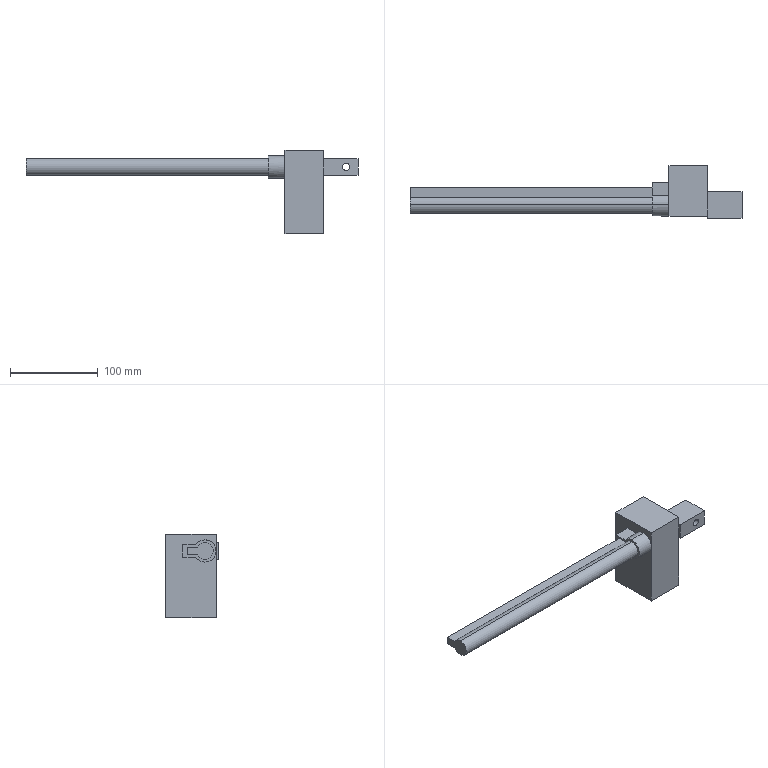Part | NX | features BREP 1 | 1 solid | 28 faces | box 379 x 59.436 x 95.25 mm | volume 383836 mm3 | plane 20 | cylinder 8 | commonest cylinder face diameters 19.304 x3 25.4 x3 8.255 x2
STEP:
#1=CARTESIAN_POINT('',(-19.05,25.4,6.985));
#2=VERTEX_POINT('',#1);
#3=CARTESIAN_POINT('',(-19.05,25.4,-6.985));
#4=VERTEX_POINT('',#3);
#5=CARTESIAN_POINT('',(-19.05,25.4,6.985));
#6=DIRECTION('',(0.,0.,-1.));
#7=VECTOR('',#6,1000.);
#8=LINE('',#5,#7);
#9=EDGE_CURVE('',#2,#4,#8,.T.);
#10=ORIENTED_EDGE('',*,*,#9,.T.);
#11=CARTESIAN_POINT('',(-19.05,10.607,-6.985));
#12=VERTEX_POINT('',#11);
#13=CARTESIAN_POINT('',(-19.05,25.4,-6.985));
#14=DIRECTION('',(0.,-1.,0.));
#15=VECTOR('',#14,1000.);
#16=LINE('',#13,#15);
#17=EDGE_CURVE('',#4,#12,#16,.T.);
#18=ORIENTED_EDGE('',*,*,#17,.T.);
#19=CARTESIAN_POINT('',(-19.05,0.,-12.7));
#20=VERTEX_POINT('',#19);
#21=CARTESIAN_POINT('',(-19.05,0.,0.));
#22=DIRECTION('',(-1.,0.,0.));
#23=DIRECTION('',(0.,0.8352,-0.55));
#24=AXIS2_PLACEMENT_3D('',#21,#22,#23);
#25=CIRCLE('',#24,12.7);
#26=EDGE_CURVE('',#12,#20,#25,.T.);
#27=ORIENTED_EDGE('',*,*,#26,.T.);
#28=CARTESIAN_POINT('',(-19.05,0.,12.7));
#29=VERTEX_POINT('',#28);
#30=CARTESIAN_POINT('',(-19.05,0.,0.));
#31=DIRECTION('',(-1.,0.,0.));
#32=DIRECTION('',(0.,0.8352,-0.55));
#33=AXIS2_PLACEMENT_3D('',#30,#31,#32);
#34=CIRCLE('',#33,12.7);
#35=EDGE_CURVE('',#20,#29,#34,.T.);
#36=ORIENTED_EDGE('',*,*,#35,.T.);
#37=CARTESIAN_POINT('',(-19.05,10.607,6.985));
#38=VERTEX_POINT('',#37);
#39=CARTESIAN_POINT('',(-19.05,0.,0.));
#40=DIRECTION('',(-1.,0.,0.));
#41=DIRECTION('',(0.,0.8352,-0.55));
#42=AXIS2_PLACEMENT_3D('',#39,#40,#41);
#43=CIRCLE('',#42,12.7);
#44=EDGE_CURVE('',#29,#38,#43,.T.);
#45=ORIENTED_EDGE('',*,*,#44,.T.);
#46=CARTESIAN_POINT('',(-19.05,10.607,6.985));
#47=DIRECTION('',(0.,1.,0.));
#48=VECTOR('',#47,1000.);
#49=LINE('',#46,#48);
#50=EDGE_CURVE('',#38,#2,#49,.T.);
#51=ORIENTED_EDGE('',*,*,#50,.T.);
#52=EDGE_LOOP('',(#10,#18,#27,#36,#45,#51));
#53=FACE_BOUND('',#52,.T.);
#54=CARTESIAN_POINT('',(-19.05,20.32,4.445));
#55=VERTEX_POINT('',#54);
#56=CARTESIAN_POINT('',(-19.05,20.32,-4.445));
#57=VERTEX_POINT('',#56);
#58=CARTESIAN_POINT('',(-19.05,20.32,4.445));
#59=DIRECTION('',(0.,0.,-1.));
#60=VECTOR('',#59,1000.);
#61=LINE('',#58,#60);
#62=EDGE_CURVE('',#55,#57,#61,.T.);
#63=ORIENTED_EDGE('',*,*,#62,.F.);
#64=CARTESIAN_POINT('',(-19.05,8.568,4.445));
#65=VERTEX_POINT('',#64);
#66=CARTESIAN_POINT('',(-19.05,8.568,4.445));
#67=DIRECTION('',(0.,1.,0.));
#68=VECTOR('',#67,1000.);
#69=LINE('',#66,#68);
#70=EDGE_CURVE('',#65,#55,#69,.T.);
#71=ORIENTED_EDGE('',*,*,#70,.F.);
#72=CARTESIAN_POINT('',(-19.05,0.,9.652));
#73=VERTEX_POINT('',#72);
#74=CARTESIAN_POINT('',(-19.05,0.,0.));
#75=DIRECTION('',(-1.,0.,0.));
#76=DIRECTION('',(0.,0.8876,-0.4605));
#77=AXIS2_PLACEMENT_3D('',#74,#75,#76);
#78=CIRCLE('',#77,9.652);
#79=EDGE_CURVE('',#73,#65,#78,.T.);
#80=ORIENTED_EDGE('',*,*,#79,.F.);
#81=CARTESIAN_POINT('',(-19.05,0.,-9.652));
#82=VERTEX_POINT('',#81);
#83=CARTESIAN_POINT('',(-19.05,0.,0.));
#84=DIRECTION('',(-1.,0.,0.));
#85=DIRECTION('',(0.,0.8876,-0.4605));
#86=AXIS2_PLACEMENT_3D('',#83,#84,#85);
#87=CIRCLE('',#86,9.652);
#88=EDGE_CURVE('',#82,#73,#87,.T.);
#89=ORIENTED_EDGE('',*,*,#88,.F.);
#90=CARTESIAN_POINT('',(-19.05,8.568,-4.445));
#91=VERTEX_POINT('',#90);
#92=CARTESIAN_POINT('',(-19.05,0.,0.));
#93=DIRECTION('',(-1.,0.,0.));
#94=DIRECTION('',(0.,0.8876,-0.4605));
#95=AXIS2_PLACEMENT_3D('',#92,#93,#94);
#96=CIRCLE('',#95,9.652);
#97=EDGE_CURVE('',#91,#82,#96,.T.);
#98=ORIENTED_EDGE('',*,*,#97,.F.);
#99=CARTESIAN_POINT('',(-19.05,20.32,-4.445));
#100=DIRECTION('',(0.,-1.,0.));
#101=VECTOR('',#100,1000.);
#102=LINE('',#99,#101);
#103=EDGE_CURVE('',#57,#91,#102,.T.);
#104=ORIENTED_EDGE('',*,*,#103,.F.);
#105=EDGE_LOOP('',(#63,#71,#80,#89,#98,#104));
#106=FACE_BOUND('',#105,.T.);
#107=CARTESIAN_POINT('',(-19.05,0.,0.));
#108=DIRECTION('',(1.,0.,0.));
#109=DIRECTION('',(0.,1.,0.));
#110=AXIS2_PLACEMENT_3D('',#107,#108,#109);
#111=PLANE('',#110);
#112=ADVANCED_FACE('',(#53,#106),#111,.F.);
#113=CARTESIAN_POINT('',(0.,25.4,6.985));
#114=VERTEX_POINT('',#113);
#115=CARTESIAN_POINT('',(-19.05,25.4,6.985));
#116=DIRECTION('',(1.,0.,0.));
#117=VECTOR('',#116,1000.);
#118=LINE('',#115,#117);
#119=EDGE_CURVE('',#2,#114,#118,.T.);
#120=ORIENTED_EDGE('',*,*,#119,.F.);
#121=ORIENTED_EDGE('',*,*,#50,.F.);
#122=CARTESIAN_POINT('',(0.,10.607,6.985));
#123=VERTEX_POINT('',#122);
#124=CARTESIAN_POINT('',(-19.05,10.607,6.985));
#125=DIRECTION('',(1.,0.,0.));
#126=VECTOR('',#125,1000.);
#127=LINE('',#124,#126);
#128=EDGE_CURVE('',#38,#123,#127,.T.);
#129=ORIENTED_EDGE('',*,*,#128,.T.);
#130=CARTESIAN_POINT('',(0.,25.4,6.985));
#131=DIRECTION('',(0.,-1.,0.));
#132=VECTOR('',#131,1000.);
#133=LINE('',#130,#132);
#134=EDGE_CURVE('',#114,#123,#133,.T.);
#135=ORIENTED_EDGE('',*,*,#134,.F.);
#136=EDGE_LOOP('',(#120,#121,#129,#135));
#137=FACE_BOUND('',#136,.T.);
#138=CARTESIAN_POINT('',(0.,25.4,6.985));
#139=DIRECTION('',(0.,0.,1.));
#140=DIRECTION('',(1.,0.,0.));
#141=AXIS2_PLACEMENT_3D('',#138,#139,#140);
#142=PLANE('',#141);
#143=ADVANCED_FACE('',(#137),#142,.T.);
#144=CARTESIAN_POINT('',(0.,0.,12.7));
#145=VERTEX_POINT('',#144);
#146=CARTESIAN_POINT('',(0.,0.,0.));
#147=DIRECTION('',(1.,0.,0.));
#148=DIRECTION('',(0.,0.8352,0.55));
#149=AXIS2_PLACEMENT_3D('',#146,#147,#148);
#150=CIRCLE('',#149,12.7);
#151=EDGE_CURVE('',#123,#145,#150,.T.);
#152=ORIENTED_EDGE('',*,*,#151,.T.);
#153=CARTESIAN_POINT('',(0.,-12.7,0.));
#154=VERTEX_POINT('',#153);
#155=CARTESIAN_POINT('',(0.,0.,0.));
#156=DIRECTION('',(1.,0.,0.));
#157=DIRECTION('',(0.,0.8352,0.55));
#158=AXIS2_PLACEMENT_3D('',#155,#156,#157);
#159=CIRCLE('',#158,12.7);
#160=EDGE_CURVE('',#145,#154,#159,.T.);
#161=ORIENTED_EDGE('',*,*,#160,.T.);
#162=CARTESIAN_POINT('',(0.,-12.7,19.05));
#163=VERTEX_POINT('',#162);
#164=CARTESIAN_POINT('',(0.,-12.7,0.));
#165=DIRECTION('',(0.,0.,1.));
#166=VECTOR('',#165,1000.);
#167=LINE('',#164,#166);
#168=EDGE_CURVE('',#154,#163,#167,.T.);
#169=ORIENTED_EDGE('',*,*,#168,.T.);
#170=CARTESIAN_POINT('',(0.,44.45,19.05));
#171=VERTEX_POINT('',#170);
#172=CARTESIAN_POINT('',(0.,44.45,19.05));
#173=DIRECTION('',(0.,-1.,0.));
#174=VECTOR('',#173,1000.);
#175=LINE('',#172,#174);
#176=EDGE_CURVE('',#171,#163,#175,.T.);
#177=ORIENTED_EDGE('',*,*,#176,.F.);
#178=CARTESIAN_POINT('',(0.,44.45,-76.2));
#179=VERTEX_POINT('',#178);
#180=CARTESIAN_POINT('',(0.,44.45,-76.2));
#181=DIRECTION('',(0.,0.,1.));
#182=VECTOR('',#181,1000.);
#183=LINE('',#180,#182);
#184=EDGE_CURVE('',#179,#171,#183,.T.);
#185=ORIENTED_EDGE('',*,*,#184,.F.);
#186=CARTESIAN_POINT('',(0.,-12.7,-76.2));
#187=VERTEX_POINT('',#186);
#188=CARTESIAN_POINT('',(0.,44.45,-76.2));
#189=DIRECTION('',(0.,-1.,0.));
#190=VECTOR('',#189,1000.);
#191=LINE('',#188,#190);
#192=EDGE_CURVE('',#179,#187,#191,.T.);
#193=ORIENTED_EDGE('',*,*,#192,.T.);
#194=CARTESIAN_POINT('',(0.,-12.7,-76.2));
#195=DIRECTION('',(0.,0.,1.));
#196=VECTOR('',#195,1000.);
#197=LINE('',#194,#196);
#198=EDGE_CURVE('',#187,#154,#197,.T.);
#199=ORIENTED_EDGE('',*,*,#198,.T.);
#200=CARTESIAN_POINT('',(0.,0.,-12.7));
#201=VERTEX_POINT('',#200);
#202=CARTESIAN_POINT('',(0.,0.,0.));
#203=DIRECTION('',(1.,0.,0.));
#204=DIRECTION('',(0.,-1.,0.));
#205=AXIS2_PLACEMENT_3D('',#202,#203,#204);
#206=CIRCLE('',#205,12.7);
#207=EDGE_CURVE('',#154,#201,#206,.T.);
#208=ORIENTED_EDGE('',*,*,#207,.T.);
#209=CARTESIAN_POINT('',(0.,10.607,-6.985));
#210=VERTEX_POINT('',#209);
#211=CARTESIAN_POINT('',(0.,0.,0.));
#212=DIRECTION('',(1.,0.,0.));
#213=DIRECTION('',(0.,-1.,0.));
#214=AXIS2_PLACEMENT_3D('',#211,#212,#213);
#215=CIRCLE('',#214,12.7);
#216=EDGE_CURVE('',#201,#210,#215,.T.);
#217=ORIENTED_EDGE('',*,*,#216,.T.);
#218=CARTESIAN_POINT('',(0.,25.4,-6.985));
#219=VERTEX_POINT('',#218);
#220=CARTESIAN_POINT('',(0.,10.607,-6.985));
#221=DIRECTION('',(0.,1.,0.));
#222=VECTOR('',#221,1000.);
#223=LINE('',#220,#222);
#224=EDGE_CURVE('',#210,#219,#223,.T.);
#225=ORIENTED_EDGE('',*,*,#224,.T.);
#226=CARTESIAN_POINT('',(0.,25.4,-6.985));
#227=DIRECTION('',(0.,0.,1.));
#228=VECTOR('',#227,1000.);
#229=LINE('',#226,#228);
#230=EDGE_CURVE('',#219,#114,#229,.T.);
#231=ORIENTED_EDGE('',*,*,#230,.T.);
#232=ORIENTED_EDGE('',*,*,#134,.T.);
#233=EDGE_LOOP('',(#152,#161,#169,#177,#185,#193,#199,#208,#217,#225,#231,#232));
#234=FACE_BOUND('',#233,.T.);
#235=CARTESIAN_POINT('',(0.,44.45,-76.2));
#236=DIRECTION('',(-1.,0.,0.));
#237=DIRECTION('',(0.,0.,1.));
#238=AXIS2_PLACEMENT_3D('',#235,#236,#237);
#239=PLANE('',#238);
#240=ADVANCED_FACE('',(#234),#239,.T.);
#241=CARTESIAN_POINT('',(-19.05,25.4,-6.985));
#242=DIRECTION('',(1.,0.,0.));
#243=VECTOR('',#242,1000.);
#244=LINE('',#241,#243);
#245=EDGE_CURVE('',#4,#219,#244,.T.);
#246=ORIENTED_EDGE('',*,*,#245,.F.);
#247=ORIENTED_EDGE('',*,*,#9,.F.);
#248=ORIENTED_EDGE('',*,*,#119,.T.);
#249=ORIENTED_EDGE('',*,*,#230,.F.);
#250=EDGE_LOOP('',(#246,#247,#248,#249));
#251=FACE_BOUND('',#250,.T.);
#252=CARTESIAN_POINT('',(0.,25.4,-6.985));
#253=DIRECTION('',(0.,1.,0.));
#254=DIRECTION('',(1.,0.,0.));
#255=AXIS2_PLACEMENT_3D('',#252,#253,#254);
#256=PLANE('',#255);
#257=ADVANCED_FACE('',(#251),#256,.T.);
#258=CARTESIAN_POINT('',(-19.05,10.607,-6.985));
#259=DIRECTION('',(1.,0.,0.));
#260=VECTOR('',#259,1000.);
#261=LINE('',#258,#260);
#262=EDGE_CURVE('',#12,#210,#261,.T.);
#263=ORIENTED_EDGE('',*,*,#262,.F.);
#264=ORIENTED_EDGE('',*,*,#17,.F.);
#265=ORIENTED_EDGE('',*,*,#245,.T.);
#266=ORIENTED_EDGE('',*,*,#224,.F.);
#267=EDGE_LOOP('',(#263,#264,#265,#266));
#268=FACE_BOUND('',#267,.T.);
#269=CARTESIAN_POINT('',(0.,10.607,-6.985));
#270=DIRECTION('',(0.,0.,-1.));
#271=DIRECTION('',(0.,-1.,0.));
#272=AXIS2_PLACEMENT_3D('',#269,#270,#271);
#273=PLANE('',#272);
#274=ADVANCED_FACE('',(#268),#273,.T.);
#275=CARTESIAN_POINT('',(0.,0.,-12.7));
#276=DIRECTION('',(1.,0.,0.));
#277=VECTOR('',#276,1000.);
#278=LINE('',#275,#277);
#279=EDGE_CURVE('',#20,#201,#278,.T.);
#280=ORIENTED_EDGE('',*,*,#279,.F.);
#281=ORIENTED_EDGE('',*,*,#26,.F.);
#282=ORIENTED_EDGE('',*,*,#262,.T.);
#283=ORIENTED_EDGE('',*,*,#216,.F.);
#284=EDGE_LOOP('',(#280,#281,#282,#283));
#285=FACE_BOUND('',#284,.T.);
#286=CARTESIAN_POINT('',(0.,0.,0.));
#287=DIRECTION('',(1.,0.,0.));
#288=DIRECTION('',(0.,0.,-1.));
#289=AXIS2_PLACEMENT_3D('',#286,#287,#288);
#290=CYLINDRICAL_SURFACE('',#289,12.7);
#291=ADVANCED_FACE('',(#285),#290,.T.);
#292=CARTESIAN_POINT('',(44.45,-12.7,9.525));
#293=VERTEX_POINT('',#292);
#294=CARTESIAN_POINT('',(44.45,-12.7,19.05));
#295=VERTEX_POINT('',#294);
#296=CARTESIAN_POINT('',(44.45,-12.7,9.525));
#297=DIRECTION('',(0.,0.,1.));
#298=VECTOR('',#297,1000.);
#299=LINE('',#296,#298);
#300=EDGE_CURVE('',#293,#295,#299,.T.);
#301=ORIENTED_EDGE('',*,*,#300,.T.);
#302=CARTESIAN_POINT('',(0.,-12.7,19.05));
#303=DIRECTION('',(1.,0.,0.));
#304=VECTOR('',#303,1000.);
#305=LINE('',#302,#304);
#306=EDGE_CURVE('',#163,#295,#305,.T.);
#307=ORIENTED_EDGE('',*,*,#306,.F.);
#308=ORIENTED_EDGE('',*,*,#168,.F.);
#309=ORIENTED_EDGE('',*,*,#198,.F.);
#310=CARTESIAN_POINT('',(44.45,-12.7,-76.2));
#311=VERTEX_POINT('',#310);
#312=CARTESIAN_POINT('',(0.,-12.7,-76.2));
#313=DIRECTION('',(1.,0.,0.));
#314=VECTOR('',#313,1000.);
#315=LINE('',#312,#314);
#316=EDGE_CURVE('',#187,#311,#315,.T.);
#317=ORIENTED_EDGE('',*,*,#316,.T.);
#318=CARTESIAN_POINT('',(44.45,-12.7,-9.525));
#319=VERTEX_POINT('',#318);
#320=CARTESIAN_POINT('',(44.45,-12.7,-76.2));
#321=DIRECTION('',(0.,0.,1.));
#322=VECTOR('',#321,1000.);
#323=LINE('',#320,#322);
#324=EDGE_CURVE('',#311,#319,#323,.T.);
#325=ORIENTED_EDGE('',*,*,#324,.T.);
#326=CARTESIAN_POINT('',(44.45,-12.7,-9.525));
#327=DIRECTION('',(0.,0.,1.));
#328=VECTOR('',#327,1000.);
#329=LINE('',#326,#328);
#330=EDGE_CURVE('',#319,#293,#329,.T.);
#331=ORIENTED_EDGE('',*,*,#330,.T.);
#332=EDGE_LOOP('',(#301,#307,#308,#309,#317,#325,#331));
#333=FACE_BOUND('',#332,.T.);
#334=CARTESIAN_POINT('',(0.,-12.7,-76.2));
#335=DIRECTION('',(0.,-1.,0.));
#336=DIRECTION('',(0.,0.,-1.));
#337=AXIS2_PLACEMENT_3D('',#334,#335,#336);
#338=PLANE('',#337);
#339=ADVANCED_FACE('',(#333),#338,.T.);
#340=CARTESIAN_POINT('',(44.45,-14.986,-9.525));
#341=VERTEX_POINT('',#340);
#342=CARTESIAN_POINT('',(44.45,-12.7,-9.525));
#343=DIRECTION('',(0.,-1.,0.));
#344=VECTOR('',#343,1000.);
#345=LINE('',#342,#344);
#346=EDGE_CURVE('',#319,#341,#345,.T.);
#347=ORIENTED_EDGE('',*,*,#346,.T.);
#348=CARTESIAN_POINT('',(44.45,-14.986,9.525));
#349=VERTEX_POINT('',#348);
#350=CARTESIAN_POINT('',(44.45,-14.986,-9.525));
#351=DIRECTION('',(0.,0.,1.));
#352=VECTOR('',#351,1000.);
#353=LINE('',#350,#352);
#354=EDGE_CURVE('',#341,#349,#353,.T.);
#355=ORIENTED_EDGE('',*,*,#354,.T.);
#356=CARTESIAN_POINT('',(44.45,-12.7,9.525));
#357=DIRECTION('',(0.,-1.,0.));
#358=VECTOR('',#357,1000.);
#359=LINE('',#356,#358);
#360=EDGE_CURVE('',#293,#349,#359,.T.);
#361=ORIENTED_EDGE('',*,*,#360,.F.);
#362=ORIENTED_EDGE('',*,*,#330,.F.);
#363=EDGE_LOOP('',(#347,#355,#361,#362));
#364=FACE_BOUND('',#363,.T.);
#365=CARTESIAN_POINT('',(44.45,14.986,-9.525));
#366=DIRECTION('',(-1.,0.,0.));
#367=DIRECTION('',(0.,0.,1.));
#368=AXIS2_PLACEMENT_3D('',#365,#366,#367);
#369=PLANE('',#368);
#370=ADVANCED_FACE('',(#364),#369,.T.);
#371=ORIENTED_EDGE('',*,*,#360,.T.);
#372=CARTESIAN_POINT('',(83.344,-14.986,9.525));
#373=VERTEX_POINT('',#372);
#374=CARTESIAN_POINT('',(44.45,-14.986,9.525));
#375=DIRECTION('',(1.,0.,0.));
#376=VECTOR('',#375,1000.);
#377=LINE('',#374,#376);
#378=EDGE_CURVE('',#349,#373,#377,.T.);
#379=ORIENTED_EDGE('',*,*,#378,.T.);
#380=CARTESIAN_POINT('',(83.344,14.986,9.525));
#381=VERTEX_POINT('',#380);
#382=CARTESIAN_POINT('',(83.344,-14.986,9.525));
#383=DIRECTION('',(0.,1.,0.));
#384=VECTOR('',#383,1000.);
#385=LINE('',#382,#384);
#386=EDGE_CURVE('',#373,#381,#385,.T.);
#387=ORIENTED_EDGE('',*,*,#386,.T.);
#388=CARTESIAN_POINT('',(44.45,14.986,9.525));
#389=VERTEX_POINT('',#388);
#390=CARTESIAN_POINT('',(83.344,14.986,9.525));
#391=DIRECTION('',(-1.,0.,0.));
#392=VECTOR('',#391,1000.);
#393=LINE('',#390,#392);
#394=EDGE_CURVE('',#381,#389,#393,.T.);
#395=ORIENTED_EDGE('',*,*,#394,.T.);
#396=CARTESIAN_POINT('',(44.45,-12.7,9.525));
#397=DIRECTION('',(0.,1.,0.));
#398=VECTOR('',#397,1000.);
#399=LINE('',#396,#398);
#400=EDGE_CURVE('',#293,#389,#399,.T.);
#401=ORIENTED_EDGE('',*,*,#400,.F.);
#402=EDGE_LOOP('',(#371,#379,#387,#395,#401));
#403=FACE_BOUND('',#402,.T.);
#404=CARTESIAN_POINT('',(0.,0.,9.525));
#405=DIRECTION('',(0.,0.,1.));
#406=DIRECTION('',(1.,0.,0.));
#407=AXIS2_PLACEMENT_3D('',#404,#405,#406);
#408=PLANE('',#407);
#409=ADVANCED_FACE('',(#403),#408,.T.);
#410=ORIENTED_EDGE('',*,*,#324,.F.);
#411=CARTESIAN_POINT('',(44.45,44.45,-76.2));
#412=VERTEX_POINT('',#411);
#413=CARTESIAN_POINT('',(44.45,-12.7,-76.2));
#414=DIRECTION('',(0.,1.,0.));
#415=VECTOR('',#414,1000.);
#416=LINE('',#413,#415);
#417=EDGE_CURVE('',#311,#412,#416,.T.);
#418=ORIENTED_EDGE('',*,*,#417,.T.);
#419=CARTESIAN_POINT('',(44.45,44.45,19.05));
#420=VERTEX_POINT('',#419);
#421=CARTESIAN_POINT('',(44.45,44.45,-76.2));
#422=DIRECTION('',(0.,0.,1.));
#423=VECTOR('',#422,1000.);
#424=LINE('',#421,#423);
#425=EDGE_CURVE('',#412,#420,#424,.T.);
#426=ORIENTED_EDGE('',*,*,#425,.T.);
#427=CARTESIAN_POINT('',(44.45,-12.7,19.05));
#428=DIRECTION('',(0.,1.,0.));
#429=VECTOR('',#428,1000.);
#430=LINE('',#427,#429);
#431=EDGE_CURVE('',#295,#420,#430,.T.);
#432=ORIENTED_EDGE('',*,*,#431,.F.);
#433=ORIENTED_EDGE('',*,*,#300,.F.);
#434=ORIENTED_EDGE('',*,*,#400,.T.);
#435=CARTESIAN_POINT('',(44.45,14.986,-9.525));
#436=VERTEX_POINT('',#435);
#437=CARTESIAN_POINT('',(44.45,14.986,-9.525));
#438=DIRECTION('',(0.,0.,1.));
#439=VECTOR('',#438,1000.);
#440=LINE('',#437,#439);
#441=EDGE_CURVE('',#436,#389,#440,.T.);
#442=ORIENTED_EDGE('',*,*,#441,.F.);
#443=CARTESIAN_POINT('',(44.45,-12.7,-9.525));
#444=DIRECTION('',(0.,1.,0.));
#445=VECTOR('',#444,1000.);
#446=LINE('',#443,#445);
#447=EDGE_CURVE('',#319,#436,#446,.T.);
#448=ORIENTED_EDGE('',*,*,#447,.F.);
#449=EDGE_LOOP('',(#410,#418,#426,#432,#433,#434,#442,#448));
#450=FACE_BOUND('',#449,.T.);
#451=CARTESIAN_POINT('',(44.45,-12.7,-76.2));
#452=DIRECTION('',(1.,0.,0.));
#453=DIRECTION('',(0.,1.,0.));
#454=AXIS2_PLACEMENT_3D('',#451,#452,#453);
#455=PLANE('',#454);
#456=ADVANCED_FACE('',(#450),#455,.T.);
#457=CARTESIAN_POINT('',(83.344,14.986,-9.525));
#458=VERTEX_POINT('',#457);
#459=CARTESIAN_POINT('',(83.344,14.986,-9.525));
#460=DIRECTION('',(-1.,0.,0.));
#461=VECTOR('',#460,1000.);
#462=LINE('',#459,#461);
#463=EDGE_CURVE('',#458,#436,#462,.T.);
#464=ORIENTED_EDGE('',*,*,#463,.F.);
#465=CARTESIAN_POINT('',(83.344,-14.986,-9.525));
#466=VERTEX_POINT('',#465);
#467=CARTESIAN_POINT('',(83.344,-14.986,-9.525));
#468=DIRECTION('',(0.,1.,0.));
#469=VECTOR('',#468,1000.);
#470=LINE('',#467,#469);
#471=EDGE_CURVE('',#466,#458,#470,.T.);
#472=ORIENTED_EDGE('',*,*,#471,.F.);
#473=CARTESIAN_POINT('',(44.45,-14.986,-9.525));
#474=DIRECTION('',(1.,0.,0.));
#475=VECTOR('',#474,1000.);
#476=LINE('',#473,#475);
#477=EDGE_CURVE('',#341,#466,#476,.T.);
#478=ORIENTED_EDGE('',*,*,#477,.F.);
#479=ORIENTED_EDGE('',*,*,#346,.F.);
#480=ORIENTED_EDGE('',*,*,#447,.T.);
#481=EDGE_LOOP('',(#464,#472,#478,#479,#480));
#482=FACE_BOUND('',#481,.T.);
#483=CARTESIAN_POINT('',(0.,0.,-9.525));
#484=DIRECTION('',(0.,0.,1.));
#485=DIRECTION('',(1.,0.,0.));
#486=AXIS2_PLACEMENT_3D('',#483,#484,#485);
#487=PLANE('',#486);
#488=ADVANCED_FACE('',(#482),#487,.F.);
#489=CARTESIAN_POINT('',(83.344,-14.986,-9.525));
#490=DIRECTION('',(0.,0.,1.));
#491=VECTOR('',#490,1000.);
#492=LINE('',#489,#491);
#493=EDGE_CURVE('',#466,#373,#492,.T.);
#494=ORIENTED_EDGE('',*,*,#493,.T.);
#495=ORIENTED_EDGE('',*,*,#378,.F.);
#496=ORIENTED_EDGE('',*,*,#354,.F.);
#497=ORIENTED_EDGE('',*,*,#477,.T.);
#498=EDGE_LOOP('',(#494,#495,#496,#497));
#499=FACE_BOUND('',#498,.T.);
#500=CARTESIAN_POINT('',(65.722,-14.986,0.));
#501=VERTEX_POINT('',#500);
#502=CARTESIAN_POINT('',(73.978,-14.986,0.));
#503=VERTEX_POINT('',#502);
#504=CARTESIAN_POINT('',(69.85,-14.986,0.));
#505=DIRECTION('',(0.,-1.,0.));
#506=DIRECTION('',(-1.,0.,0.));
#507=AXIS2_PLACEMENT_3D('',#504,#505,#506);
#508=CIRCLE('',#507,4.128);
#509=EDGE_CURVE('',#501,#503,#508,.T.);
#510=ORIENTED_EDGE('',*,*,#509,.F.);
#511=CARTESIAN_POINT('',(69.85,-14.986,0.));
#512=DIRECTION('',(0.,-1.,0.));
#513=DIRECTION('',(1.,0.,0.));
#514=AXIS2_PLACEMENT_3D('',#511,#512,#513);
#515=CIRCLE('',#514,4.128);
#516=EDGE_CURVE('',#503,#501,#515,.T.);
#517=ORIENTED_EDGE('',*,*,#516,.F.);
#518=EDGE_LOOP('',(#510,#517));
#519=FACE_BOUND('',#518,.T.);
#520=CARTESIAN_POINT('',(44.45,-14.986,-9.525));
#521=DIRECTION('',(0.,-1.,0.));
#522=DIRECTION('',(0.,0.,-1.));
#523=AXIS2_PLACEMENT_3D('',#520,#521,#522);
#524=PLANE('',#523);
#525=ADVANCED_FACE('',(#499,#519),#524,.T.);
#526=CARTESIAN_POINT('',(83.344,14.986,-9.525));
#527=DIRECTION('',(0.,0.,1.));
#528=VECTOR('',#527,1000.);
#529=LINE('',#526,#528);
#530=EDGE_CURVE('',#458,#381,#529,.T.);
#531=ORIENTED_EDGE('',*,*,#530,.T.);
#532=ORIENTED_EDGE('',*,*,#386,.F.);
#533=ORIENTED_EDGE('',*,*,#493,.F.);
#534=ORIENTED_EDGE('',*,*,#471,.T.);
#535=EDGE_LOOP('',(#531,#532,#533,#534));
#536=FACE_BOUND('',#535,.T.);
#537=CARTESIAN_POINT('',(83.344,-14.986,-9.525));
#538=DIRECTION('',(1.,0.,0.));
#539=DIRECTION('',(0.,1.,0.));
#540=AXIS2_PLACEMENT_3D('',#537,#538,#539);
#541=PLANE('',#540);
#542=ADVANCED_FACE('',(#536),#541,.T.);
#543=ORIENTED_EDGE('',*,*,#394,.F.);
#544=ORIENTED_EDGE('',*,*,#530,.F.);
#545=ORIENTED_EDGE('',*,*,#463,.T.);
#546=ORIENTED_EDGE('',*,*,#441,.T.);
#547=EDGE_LOOP('',(#543,#544,#545,#546));
#548=FACE_BOUND('',#547,.T.);
#549=CARTESIAN_POINT('',(65.722,14.986,0.));
#550=VERTEX_POINT('',#549);
#551=CARTESIAN_POINT('',(73.978,14.986,0.));
#552=VERTEX_POINT('',#551);
#553=CARTESIAN_POINT('',(69.85,14.986,0.));
#554=DIRECTION('',(0.,-1.,0.));
#555=DIRECTION('',(-1.,0.,0.));
#556=AXIS2_PLACEMENT_3D('',#553,#554,#555);
#557=CIRCLE('',#556,4.128);
#558=EDGE_CURVE('',#550,#552,#557,.T.);
#559=ORIENTED_EDGE('',*,*,#558,.T.);
#560=CARTESIAN_POINT('',(69.85,14.986,0.));
#561=DIRECTION('',(0.,-1.,0.));
#562=DIRECTION('',(1.,0.,0.));
#563=AXIS2_PLACEMENT_3D('',#560,#561,#562);
#564=CIRCLE('',#563,4.128);
#565=EDGE_CURVE('',#552,#550,#564,.T.);
#566=ORIENTED_EDGE('',*,*,#565,.T.);
#567=EDGE_LOOP('',(#559,#566));
#568=FACE_BOUND('',#567,.T.);
#569=CARTESIAN_POINT('',(83.344,14.986,-9.525));
#570=DIRECTION('',(0.,1.,0.));
#571=DIRECTION('',(1.,0.,0.));
#572=AXIS2_PLACEMENT_3D('',#569,#570,#571);
#573=PLANE('',#572);
#574=ADVANCED_FACE('',(#548,#568),#573,.T.);
#575=ORIENTED_EDGE('',*,*,#516,.T.);
#576=CARTESIAN_POINT('',(65.722,14.986,0.));
#577=DIRECTION('',(0.,-1.,0.));
#578=VECTOR('',#577,1000.);
#579=LINE('',#576,#578);
#580=EDGE_CURVE('',#501,#550,#579,.F.);
#581=ORIENTED_EDGE('',*,*,#580,.T.);
#582=ORIENTED_EDGE('',*,*,#565,.F.);
#583=CARTESIAN_POINT('',(73.978,14.986,0.));
#584=DIRECTION('',(0.,-1.,0.));
#585=VECTOR('',#584,1000.);
#586=LINE('',#583,#585);
#587=EDGE_CURVE('',#503,#552,#586,.F.);
#588=ORIENTED_EDGE('',*,*,#587,.F.);
#589=EDGE_LOOP('',(#575,#581,#582,#588));
#590=FACE_BOUND('',#589,.T.);
#591=CARTESIAN_POINT('',(69.85,14.986,0.));
#592=DIRECTION('',(0.,-1.,0.));
#593=DIRECTION('',(1.,0.,0.));
#594=AXIS2_PLACEMENT_3D('',#591,#592,#593);
#595=CYLINDRICAL_SURFACE('',#594,4.128);
#596=ADVANCED_FACE('',(#590),#595,.F.);
#597=ORIENTED_EDGE('',*,*,#558,.F.);
#598=ORIENTED_EDGE('',*,*,#580,.F.);
#599=ORIENTED_EDGE('',*,*,#509,.T.);
#600=ORIENTED_EDGE('',*,*,#587,.T.);
#601=EDGE_LOOP('',(#597,#598,#599,#600));
#602=FACE_BOUND('',#601,.T.);
#603=CARTESIAN_POINT('',(69.85,14.986,0.));
#604=DIRECTION('',(0.,-1.,0.));
#605=DIRECTION('',(1.,0.,0.));
#606=AXIS2_PLACEMENT_3D('',#603,#604,#605);
#607=CYLINDRICAL_SURFACE('',#606,4.128);
#608=ADVANCED_FACE('',(#602),#607,.F.);
#609=ORIENTED_EDGE('',*,*,#306,.T.);
#610=ORIENTED_EDGE('',*,*,#431,.T.);
#611=CARTESIAN_POINT('',(44.45,44.45,19.05));
#612=DIRECTION('',(-1.,0.,0.));
#613=VECTOR('',#612,1000.);
#614=LINE('',#611,#613);
#615=EDGE_CURVE('',#420,#171,#614,.T.);
#616=ORIENTED_EDGE('',*,*,#615,.T.);
#617=ORIENTED_EDGE('',*,*,#176,.T.);
#618=EDGE_LOOP('',(#609,#610,#616,#617));
#619=FACE_BOUND('',#618,.T.);
#620=CARTESIAN_POINT('',(0.,0.,19.05));
#621=DIRECTION('',(0.,0.,1.));
#622=DIRECTION('',(1.,0.,0.));
#623=AXIS2_PLACEMENT_3D('',#620,#621,#622);
#624=PLANE('',#623);
#625=ADVANCED_FACE('',(#619),#624,.T.);
#626=ORIENTED_EDGE('',*,*,#184,.T.);
#627=ORIENTED_EDGE('',*,*,#615,.F.);
#628=ORIENTED_EDGE('',*,*,#425,.F.);
#629=CARTESIAN_POINT('',(44.45,44.45,-76.2));
#630=DIRECTION('',(-1.,0.,0.));
#631=VECTOR('',#630,1000.);
#632=LINE('',#629,#631);
#633=EDGE_CURVE('',#412,#179,#632,.T.);
#634=ORIENTED_EDGE('',*,*,#633,.T.);
#635=EDGE_LOOP('',(#626,#627,#628,#634));
#636=FACE_BOUND('',#635,.T.);
#637=CARTESIAN_POINT('',(44.45,44.45,-76.2));
#638=DIRECTION('',(0.,1.,0.));
#639=DIRECTION('',(1.,0.,0.));
#640=AXIS2_PLACEMENT_3D('',#637,#638,#639);
#641=PLANE('',#640);
#642=ADVANCED_FACE('',(#636),#641,.T.);
#643=ORIENTED_EDGE('',*,*,#633,.F.);
#644=ORIENTED_EDGE('',*,*,#417,.F.);
#645=ORIENTED_EDGE('',*,*,#316,.F.);
#646=ORIENTED_EDGE('',*,*,#192,.F.);
#647=EDGE_LOOP('',(#643,#644,#645,#646));
#648=FACE_BOUND('',#647,.T.);
#649=CARTESIAN_POINT('',(0.,0.,-76.2));
#650=DIRECTION('',(0.,0.,1.));
#651=DIRECTION('',(1.,0.,0.));
#652=AXIS2_PLACEMENT_3D('',#649,#650,#651);
#653=PLANE('',#652);
#654=ADVANCED_FACE('',(#648),#653,.F.);
#655=CARTESIAN_POINT('',(-295.656,8.568,-4.445));
#656=VERTEX_POINT('',#655);
#657=CARTESIAN_POINT('',(-19.05,8.568,-4.445));
#658=DIRECTION('',(-1.,0.,0.));
#659=VECTOR('',#658,1000.);
#660=LINE('',#657,#659);
#661=EDGE_CURVE('',#91,#656,#660,.T.);
#662=ORIENTED_EDGE('',*,*,#661,.T.);
#663=CARTESIAN_POINT('',(-295.656,20.32,-4.445));
#664=VERTEX_POINT('',#663);
#665=CARTESIAN_POINT('',(-295.656,20.32,-4.445));
#666=DIRECTION('',(0.,-1.,0.));
#667=VECTOR('',#666,1000.);
#668=LINE('',#665,#667);
#669=EDGE_CURVE('',#664,#656,#668,.T.);
#670=ORIENTED_EDGE('',*,*,#669,.F.);
#671=CARTESIAN_POINT('',(-19.05,20.32,-4.445));
#672=DIRECTION('',(-1.,0.,0.));
#673=VECTOR('',#672,1000.);
#674=LINE('',#671,#673);
#675=EDGE_CURVE('',#57,#664,#674,.T.);
#676=ORIENTED_EDGE('',*,*,#675,.F.);
#677=ORIENTED_EDGE('',*,*,#103,.T.);
#678=EDGE_LOOP('',(#662,#670,#676,#677));
#679=FACE_BOUND('',#678,.T.);
#680=CARTESIAN_POINT('',(-19.05,20.32,-4.445));
#681=DIRECTION('',(0.,0.,-1.));
#682=DIRECTION('',(0.,-1.,0.));
#683=AXIS2_PLACEMENT_3D('',#680,#681,#682);
#684=PLANE('',#683);
#685=ADVANCED_FACE('',(#679),#684,.T.);
#686=ORIENTED_EDGE('',*,*,#675,.T.);
#687=CARTESIAN_POINT('',(-295.656,20.32,4.445));
#688=VERTEX_POINT('',#687);
#689=CARTESIAN_POINT('',(-295.656,20.32,4.445));
#690=DIRECTION('',(0.,0.,-1.));
#691=VECTOR('',#690,1000.);
#692=LINE('',#689,#691);
#693=EDGE_CURVE('',#688,#664,#692,.T.);
#694=ORIENTED_EDGE('',*,*,#693,.F.);
#695=CARTESIAN_POINT('',(-19.05,20.32,4.445));
#696=DIRECTION('',(-1.,0.,0.));
#697=VECTOR('',#696,1000.);
#698=LINE('',#695,#697);
#699=EDGE_CURVE('',#55,#688,#698,.T.);
#700=ORIENTED_EDGE('',*,*,#699,.F.);
#701=ORIENTED_EDGE('',*,*,#62,.T.);
#702=EDGE_LOOP('',(#686,#694,#700,#701));
#703=FACE_BOUND('',#702,.T.);
#704=CARTESIAN_POINT('',(-19.05,20.32,4.445));
#705=DIRECTION('',(0.,1.,0.));
#706=DIRECTION('',(1.,0.,0.));
#707=AXIS2_PLACEMENT_3D('',#704,#705,#706);
#708=PLANE('',#707);
#709=ADVANCED_FACE('',(#703),#708,.T.);
#710=ORIENTED_EDGE('',*,*,#699,.T.);
#711=CARTESIAN_POINT('',(-295.656,8.568,4.445));
#712=VERTEX_POINT('',#711);
#713=CARTESIAN_POINT('',(-295.656,8.568,4.445));
#714=DIRECTION('',(0.,1.,0.));
#715=VECTOR('',#714,1000.);
#716=LINE('',#713,#715);
#717=EDGE_CURVE('',#712,#688,#716,.T.);
#718=ORIENTED_EDGE('',*,*,#717,.F.);
#719=CARTESIAN_POINT('',(-19.05,8.568,4.445));
#720=DIRECTION('',(-1.,0.,0.));
#721=VECTOR('',#720,1000.);
#722=LINE('',#719,#721);
#723=EDGE_CURVE('',#65,#712,#722,.T.);
#724=ORIENTED_EDGE('',*,*,#723,.F.);
#725=ORIENTED_EDGE('',*,*,#70,.T.);
#726=EDGE_LOOP('',(#710,#718,#724,#725));
#727=FACE_BOUND('',#726,.T.);
#728=CARTESIAN_POINT('',(-19.05,8.568,4.445));
#729=DIRECTION('',(0.,0.,1.));
#730=DIRECTION('',(1.,0.,0.));
#731=AXIS2_PLACEMENT_3D('',#728,#729,#730);
#732=PLANE('',#731);
#733=ADVANCED_FACE('',(#727),#732,.T.);
#734=CARTESIAN_POINT('',(-295.656,0.,9.652));
#735=VERTEX_POINT('',#734);
#736=CARTESIAN_POINT('',(-19.05,0.,9.652));
#737=DIRECTION('',(-1.,0.,0.));
#738=VECTOR('',#737,1000.);
#739=LINE('',#736,#738);
#740=EDGE_CURVE('',#73,#735,#739,.T.);
#741=ORIENTED_EDGE('',*,*,#740,.F.);
#742=ORIENTED_EDGE('',*,*,#79,.T.);
#743=ORIENTED_EDGE('',*,*,#723,.T.);
#744=CARTESIAN_POINT('',(-295.656,0.,0.));
#745=DIRECTION('',(-1.,0.,0.));
#746=DIRECTION('',(0.,0.8876,-0.4605));
#747=AXIS2_PLACEMENT_3D('',#744,#745,#746);
#748=CIRCLE('',#747,9.652);
#749=EDGE_CURVE('',#735,#712,#748,.T.);
#750=ORIENTED_EDGE('',*,*,#749,.F.);
#751=EDGE_LOOP('',(#741,#742,#743,#750));
#752=FACE_BOUND('',#751,.T.);
#753=CARTESIAN_POINT('',(-19.05,0.,0.));
#754=DIRECTION('',(-1.,0.,0.));
#755=DIRECTION('',(0.,0.,1.));
#756=AXIS2_PLACEMENT_3D('',#753,#754,#755);
#757=CYLINDRICAL_SURFACE('',#756,9.652);
#758=ADVANCED_FACE('',(#752),#757,.T.);
#759=CARTESIAN_POINT('',(-295.656,0.,-9.652));
#760=VERTEX_POINT('',#759);
#761=CARTESIAN_POINT('',(-295.656,0.,0.));
#762=DIRECTION('',(-1.,0.,0.));
#763=DIRECTION('',(0.,0.8876,-0.4605));
#764=AXIS2_PLACEMENT_3D('',#761,#762,#763);
#765=CIRCLE('',#764,9.652);
#766=EDGE_CURVE('',#656,#760,#765,.T.);
#767=ORIENTED_EDGE('',*,*,#766,.T.);
#768=CARTESIAN_POINT('',(-295.656,0.,0.));
#769=DIRECTION('',(-1.,0.,0.));
#770=DIRECTION('',(0.,0.8876,-0.4605));
#771=AXIS2_PLACEMENT_3D('',#768,#769,#770);
#772=CIRCLE('',#771,9.652);
#773=EDGE_CURVE('',#760,#735,#772,.T.);
#774=ORIENTED_EDGE('',*,*,#773,.T.);
#775=ORIENTED_EDGE('',*,*,#749,.T.);
#776=ORIENTED_EDGE('',*,*,#717,.T.);
#777=ORIENTED_EDGE('',*,*,#693,.T.);
#778=ORIENTED_EDGE('',*,*,#669,.T.);
#779=EDGE_LOOP('',(#767,#774,#775,#776,#777,#778));
#780=FACE_BOUND('',#779,.T.);
#781=CARTESIAN_POINT('',(-295.656,14.986,0.));
#782=DIRECTION('',(1.,0.,0.));
#783=DIRECTION('',(0.,1.,0.));
#784=AXIS2_PLACEMENT_3D('',#781,#782,#783);
#785=PLANE('',#784);
#786=ADVANCED_FACE('',(#780),#785,.F.);
#787=CARTESIAN_POINT('',(-19.05,0.,-9.652));
#788=DIRECTION('',(-1.,0.,0.));
#789=VECTOR('',#788,1000.);
#790=LINE('',#787,#789);
#791=EDGE_CURVE('',#82,#760,#790,.T.);
#792=ORIENTED_EDGE('',*,*,#791,.F.);
#793=ORIENTED_EDGE('',*,*,#88,.T.);
#794=ORIENTED_EDGE('',*,*,#740,.T.);
#795=ORIENTED_EDGE('',*,*,#773,.F.);
#796=EDGE_LOOP('',(#792,#793,#794,#795));
#797=FACE_BOUND('',#796,.T.);
#798=CARTESIAN_POINT('',(-19.05,0.,0.));
#799=DIRECTION('',(-1.,0.,0.));
#800=DIRECTION('',(0.,0.,1.));
#801=AXIS2_PLACEMENT_3D('',#798,#799,#800);
#802=CYLINDRICAL_SURFACE('',#801,9.652);
#803=ADVANCED_FACE('',(#797),#802,.T.);
#804=ORIENTED_EDGE('',*,*,#97,.T.);
#805=ORIENTED_EDGE('',*,*,#791,.T.);
#806=ORIENTED_EDGE('',*,*,#766,.F.);
#807=ORIENTED_EDGE('',*,*,#661,.F.);
#808=EDGE_LOOP('',(#804,#805,#806,#807));
#809=FACE_BOUND('',#808,.T.);
#810=CARTESIAN_POINT('',(-19.05,0.,0.));
#811=DIRECTION('',(-1.,0.,0.));
#812=DIRECTION('',(0.,0.,1.));
#813=AXIS2_PLACEMENT_3D('',#810,#811,#812);
#814=CYLINDRICAL_SURFACE('',#813,9.652);
#815=ADVANCED_FACE('',(#809),#814,.T.);
#816=CARTESIAN_POINT('',(0.,0.,12.7));
#817=DIRECTION('',(1.,0.,0.));
#818=VECTOR('',#817,1000.);
#819=LINE('',#816,#818);
#820=EDGE_CURVE('',#29,#145,#819,.T.);
#821=ORIENTED_EDGE('',*,*,#820,.F.);
#822=ORIENTED_EDGE('',*,*,#35,.F.);
#823=ORIENTED_EDGE('',*,*,#279,.T.);
#824=ORIENTED_EDGE('',*,*,#207,.F.);
#825=ORIENTED_EDGE('',*,*,#160,.F.);
#826=EDGE_LOOP('',(#821,#822,#823,#824,#825));
#827=FACE_BOUND('',#826,.T.);
#828=CARTESIAN_POINT('',(0.,0.,0.));
#829=DIRECTION('',(1.,0.,0.));
#830=DIRECTION('',(0.,0.,-1.));
#831=AXIS2_PLACEMENT_3D('',#828,#829,#830);
#832=CYLINDRICAL_SURFACE('',#831,12.7);
#833=ADVANCED_FACE('',(#827),#832,.T.);
#834=ORIENTED_EDGE('',*,*,#44,.F.);
#835=ORIENTED_EDGE('',*,*,#820,.T.);
#836=ORIENTED_EDGE('',*,*,#151,.F.);
#837=ORIENTED_EDGE('',*,*,#128,.F.);
#838=EDGE_LOOP('',(#834,#835,#836,#837));
#839=FACE_BOUND('',#838,.T.);
#840=CARTESIAN_POINT('',(0.,0.,0.));
#841=DIRECTION('',(1.,0.,0.));
#842=DIRECTION('',(0.,0.,-1.));
#843=AXIS2_PLACEMENT_3D('',#840,#841,#842);
#844=CYLINDRICAL_SURFACE('',#843,12.7);
#845=ADVANCED_FACE('',(#839),#844,.T.);
#846=CLOSED_SHELL('',(#112,#143,#240,#257,#274,#291,#339,#370,#409,#456,#488,#525,#542,#574,#596,#608,#625,#642,#654,#685,#709,#733,#758,#786,#803,#815,#833,#845));
#847=MANIFOLD_SOLID_BREP('',#846);
#848=(LENGTH_UNIT()NAMED_UNIT(*)SI_UNIT(.MILLI.,.METRE.));
#849=UNCERTAINTY_MEASURE_WITH_UNIT(LENGTH_MEASURE(0.00001),#848,'','');
#850=(NAMED_UNIT(*)PLANE_ANGLE_UNIT()SI_UNIT($,.RADIAN.));
#851=(NAMED_UNIT(*)SI_UNIT($,.STERADIAN.)SOLID_ANGLE_UNIT());
#852=(GEOMETRIC_REPRESENTATION_CONTEXT(3)GLOBAL_UNCERTAINTY_ASSIGNED_CONTEXT((#849))GLOBAL_UNIT_ASSIGNED_CONTEXT((#848,#850,#851))REPRESENTATION_CONTEXT('',''));
#853=ADVANCED_BREP_SHAPE_REPRESENTATION('',(#847),#852);